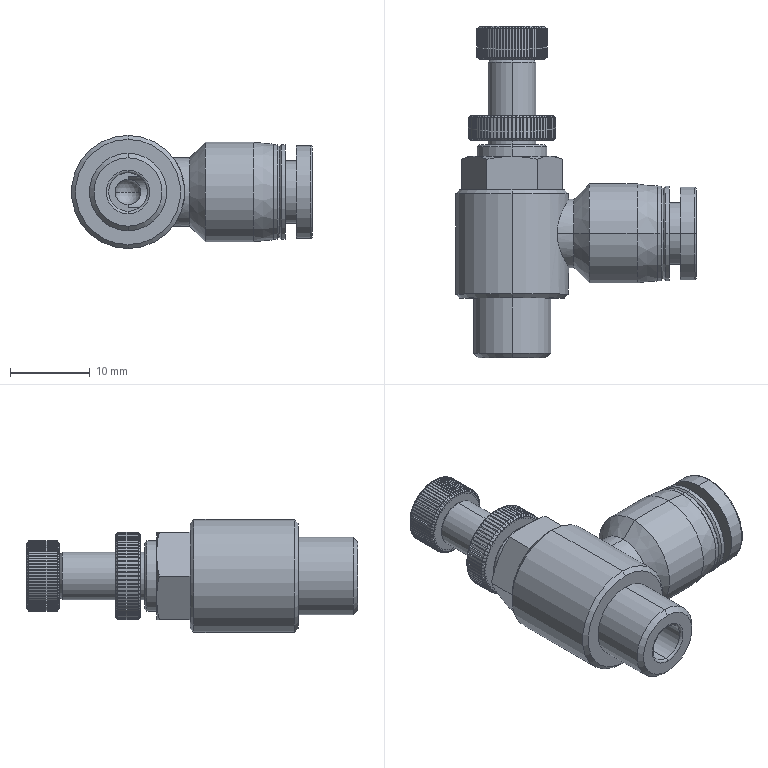Part | STEP file | Exhaust throttle valve PSL601A | 1 solid | 820 faces | box 30.2 x 41.6 x 14.2 mm | volume 4827 mm3 | plane 323 | cone 312 | cylinder 177 | torus 6 | sphere 2 | commonest cylinder face diameters 8.8 x74 11 x72 6 x6 11.9 x4 3.243 x3 4 x2